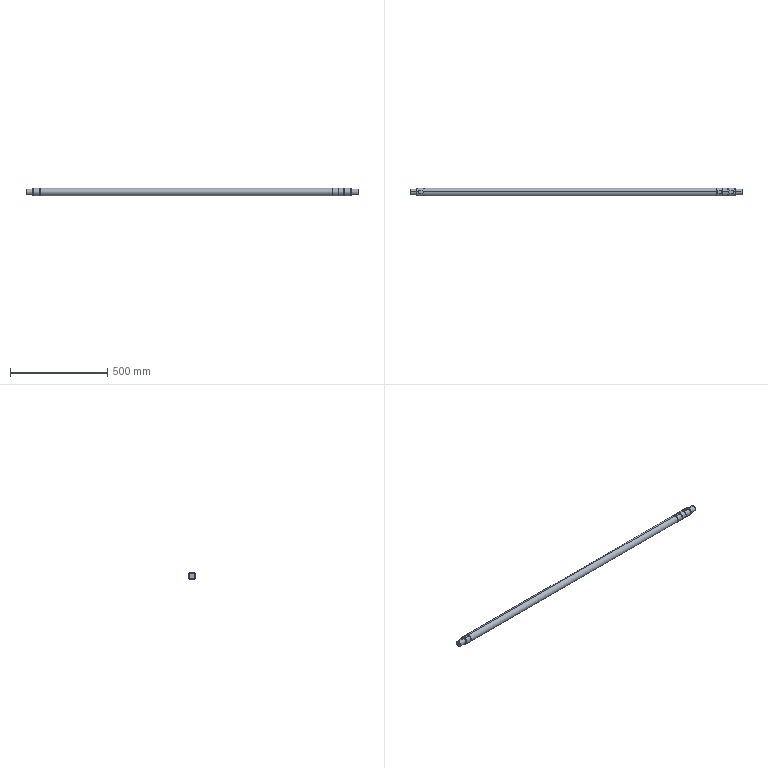Part | SolidWorks | features ICE 3, RevCut 2, Extrusion 1, LPattern 1 | 1 solid | 64 faces | box 1705 x 40 x 40 mm | volume 2098690 mm3 | cylinder 39 | plane 25 | commonest cylinder face diameters 40 x14 37.5 x12 12 x9 30 x4